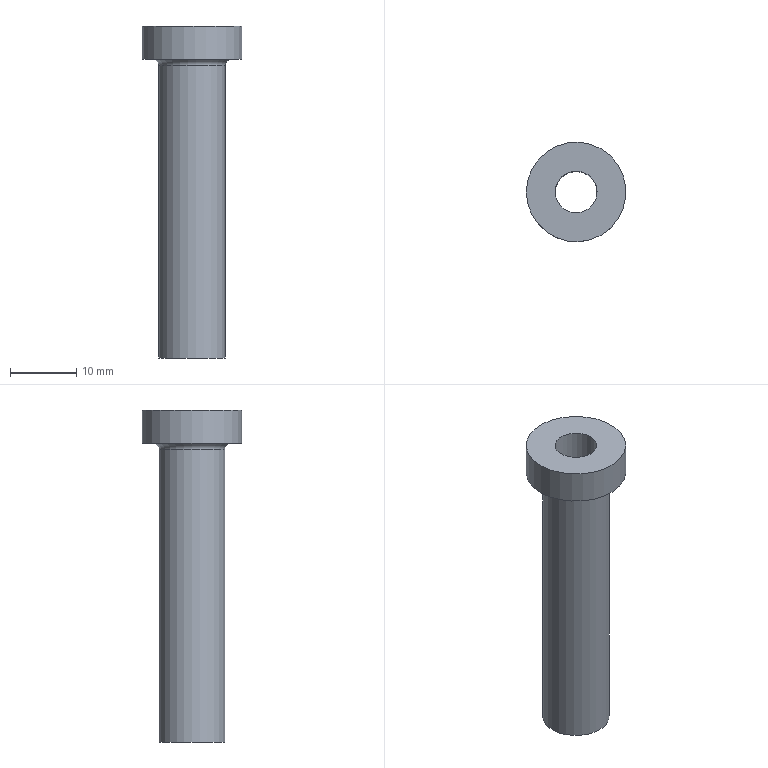Part | NX | features PG_666 2 | 1 solid | 7 faces | box 15 x 15 x 50 mm | volume 2866 mm3 | plane 3 | cylinder 3 | torus 1 | commonest cylinder face diameters 6.3 x1 10 x1 15 x1
STEP:
#1=CARTESIAN_POINT('',(3986.944,-923.622,803.716));
#2=VERTEX_POINT('',#1);
#3=CARTESIAN_POINT('',(3990.094,-923.622,803.716));
#4=DIRECTION('',(0.,0.,-1.));
#5=DIRECTION('',(-1.,0.,0.));
#6=AXIS2_PLACEMENT_3D('',#3,#4,#5);
#7=CIRCLE('',#6,3.15);
#8=EDGE_CURVE('',#2,#2,#7,.T.);
#9=ORIENTED_EDGE('',*,*,#8,.F.);
#10=EDGE_LOOP('',(#9));
#11=FACE_BOUND('',#10,.T.);
#12=CARTESIAN_POINT('',(3985.094,-923.622,803.716));
#13=VERTEX_POINT('',#12);
#14=CARTESIAN_POINT('',(3990.094,-923.622,803.716));
#15=DIRECTION('',(0.,0.,-1.));
#16=DIRECTION('',(-1.,0.,0.));
#17=AXIS2_PLACEMENT_3D('',#14,#15,#16);
#18=CIRCLE('',#17,5.);
#19=EDGE_CURVE('',#13,#13,#18,.T.);
#20=ORIENTED_EDGE('',*,*,#19,.T.);
#21=EDGE_LOOP('',(#20));
#22=FACE_BOUND('',#21,.T.);
#23=CARTESIAN_POINT('',(3990.094,-923.622,803.716));
#24=DIRECTION('',(0.,0.,-1.));
#25=DIRECTION('',(1.,0.,0.));
#26=AXIS2_PLACEMENT_3D('',#23,#24,#25);
#27=PLANE('',#26);
#28=ADVANCED_FACE('',(#11,#22),#27,.T.);
#29=CARTESIAN_POINT('',(3995.094,-923.622,847.716));
#30=VERTEX_POINT('',#29);
#31=CARTESIAN_POINT('',(3990.094,-923.622,847.716));
#32=DIRECTION('',(0.,0.,1.));
#33=DIRECTION('',(1.,0.,0.));
#34=AXIS2_PLACEMENT_3D('',#31,#32,#33);
#35=CIRCLE('',#34,5.);
#36=EDGE_CURVE('',#30,#30,#35,.T.);
#37=ORIENTED_EDGE('',*,*,#36,.F.);
#38=EDGE_LOOP('',(#37));
#39=FACE_BOUND('',#38,.T.);
#40=ORIENTED_EDGE('',*,*,#19,.F.);
#41=EDGE_LOOP('',(#40));
#42=FACE_BOUND('',#41,.T.);
#43=CARTESIAN_POINT('',(3990.094,-923.622,823.716));
#44=DIRECTION('',(0.,0.,1.));
#45=DIRECTION('',(-1.,0.,0.));
#46=AXIS2_PLACEMENT_3D('',#43,#44,#45);
#47=CYLINDRICAL_SURFACE('',#46,5.);
#48=ADVANCED_FACE('',(#39,#42),#47,.T.);
#49=CARTESIAN_POINT('',(3986.944,-923.622,853.716));
#50=VERTEX_POINT('',#49);
#51=CARTESIAN_POINT('',(3990.094,-923.622,853.716));
#52=DIRECTION('',(0.,0.,-1.));
#53=DIRECTION('',(-1.,0.,0.));
#54=AXIS2_PLACEMENT_3D('',#51,#52,#53);
#55=CIRCLE('',#54,3.15);
#56=EDGE_CURVE('',#50,#50,#55,.F.);
#57=ORIENTED_EDGE('',*,*,#56,.F.);
#58=EDGE_LOOP('',(#57));
#59=FACE_BOUND('',#58,.T.);
#60=CARTESIAN_POINT('',(3982.594,-923.622,853.716));
#61=VERTEX_POINT('',#60);
#62=CARTESIAN_POINT('',(3990.094,-923.622,853.716));
#63=DIRECTION('',(0.,0.,1.));
#64=DIRECTION('',(-1.,0.,0.));
#65=AXIS2_PLACEMENT_3D('',#62,#63,#64);
#66=CIRCLE('',#65,7.5);
#67=EDGE_CURVE('',#61,#61,#66,.T.);
#68=ORIENTED_EDGE('',*,*,#67,.T.);
#69=EDGE_LOOP('',(#68));
#70=FACE_BOUND('',#69,.T.);
#71=CARTESIAN_POINT('',(3990.094,-923.622,853.716));
#72=DIRECTION('',(0.,0.,1.));
#73=DIRECTION('',(-1.,0.,0.));
#74=AXIS2_PLACEMENT_3D('',#71,#72,#73);
#75=PLANE('',#74);
#76=ADVANCED_FACE('',(#59,#70),#75,.T.);
#77=CARTESIAN_POINT('',(3996.094,-923.622,848.716));
#78=VERTEX_POINT('',#77);
#79=CARTESIAN_POINT('',(3990.094,-923.622,848.716));
#80=DIRECTION('',(0.,0.,1.));
#81=DIRECTION('',(1.,0.,0.));
#82=AXIS2_PLACEMENT_3D('',#79,#80,#81);
#83=CIRCLE('',#82,6.);
#84=EDGE_CURVE('',#78,#78,#83,.F.);
#85=ORIENTED_EDGE('',*,*,#84,.F.);
#86=EDGE_LOOP('',(#85));
#87=FACE_BOUND('',#86,.T.);
#88=CARTESIAN_POINT('',(3982.594,-923.622,848.716));
#89=VERTEX_POINT('',#88);
#90=CARTESIAN_POINT('',(3990.094,-923.622,848.716));
#91=DIRECTION('',(0.,0.,-1.));
#92=DIRECTION('',(-1.,0.,0.));
#93=AXIS2_PLACEMENT_3D('',#90,#91,#92);
#94=CIRCLE('',#93,7.5);
#95=EDGE_CURVE('',#89,#89,#94,.T.);
#96=ORIENTED_EDGE('',*,*,#95,.T.);
#97=EDGE_LOOP('',(#96));
#98=FACE_BOUND('',#97,.T.);
#99=CARTESIAN_POINT('',(3990.094,-923.622,848.716));
#100=DIRECTION('',(0.,0.,-1.));
#101=DIRECTION('',(1.,0.,0.));
#102=AXIS2_PLACEMENT_3D('',#99,#100,#101);
#103=PLANE('',#102);
#104=ADVANCED_FACE('',(#87,#98),#103,.T.);
#105=ORIENTED_EDGE('',*,*,#67,.F.);
#106=EDGE_LOOP('',(#105));
#107=FACE_BOUND('',#106,.T.);
#108=ORIENTED_EDGE('',*,*,#95,.F.);
#109=EDGE_LOOP('',(#108));
#110=FACE_BOUND('',#109,.T.);
#111=CARTESIAN_POINT('',(3990.094,-923.622,848.716));
#112=DIRECTION('',(0.,0.,1.));
#113=DIRECTION('',(-1.,0.,0.));
#114=AXIS2_PLACEMENT_3D('',#111,#112,#113);
#115=CYLINDRICAL_SURFACE('',#114,7.5);
#116=ADVANCED_FACE('',(#107,#110),#115,.T.);
#117=ORIENTED_EDGE('',*,*,#56,.T.);
#118=EDGE_LOOP('',(#117));
#119=FACE_BOUND('',#118,.T.);
#120=ORIENTED_EDGE('',*,*,#8,.T.);
#121=EDGE_LOOP('',(#120));
#122=FACE_BOUND('',#121,.T.);
#123=CARTESIAN_POINT('',(3990.094,-923.622,823.716));
#124=DIRECTION('',(0.,0.,1.));
#125=DIRECTION('',(-1.,0.,0.));
#126=AXIS2_PLACEMENT_3D('',#123,#124,#125);
#127=CYLINDRICAL_SURFACE('',#126,3.15);
#128=ADVANCED_FACE('',(#119,#122),#127,.F.);
#129=ORIENTED_EDGE('',*,*,#36,.T.);
#130=EDGE_LOOP('',(#129));
#131=FACE_BOUND('',#130,.T.);
#132=ORIENTED_EDGE('',*,*,#84,.T.);
#133=EDGE_LOOP('',(#132));
#134=FACE_BOUND('',#133,.T.);
#135=CARTESIAN_POINT('',(3990.094,-923.622,847.716));
#136=DIRECTION('',(0.,0.,-1.));
#137=DIRECTION('',(1.,0.,0.));
#138=AXIS2_PLACEMENT_3D('',#135,#136,#137);
#139=TOROIDAL_SURFACE('',#138,6.,1.);
#140=ADVANCED_FACE('',(#131,#134),#139,.F.);
#141=CLOSED_SHELL('',(#28,#48,#76,#104,#116,#128,#140));
#142=MANIFOLD_SOLID_BREP('',#141);
#143=(LENGTH_UNIT()NAMED_UNIT(*)SI_UNIT(.MILLI.,.METRE.));
#144=UNCERTAINTY_MEASURE_WITH_UNIT(LENGTH_MEASURE(0.00001),#143,'','');
#145=(NAMED_UNIT(*)PLANE_ANGLE_UNIT()SI_UNIT($,.RADIAN.));
#146=(NAMED_UNIT(*)SI_UNIT($,.STERADIAN.)SOLID_ANGLE_UNIT());
#147=(GEOMETRIC_REPRESENTATION_CONTEXT(3)GLOBAL_UNCERTAINTY_ASSIGNED_CONTEXT((#144))GLOBAL_UNIT_ASSIGNED_CONTEXT((#143,#145,#146))REPRESENTATION_CONTEXT('',''));
#148=ADVANCED_BREP_SHAPE_REPRESENTATION('',(#142),#147);